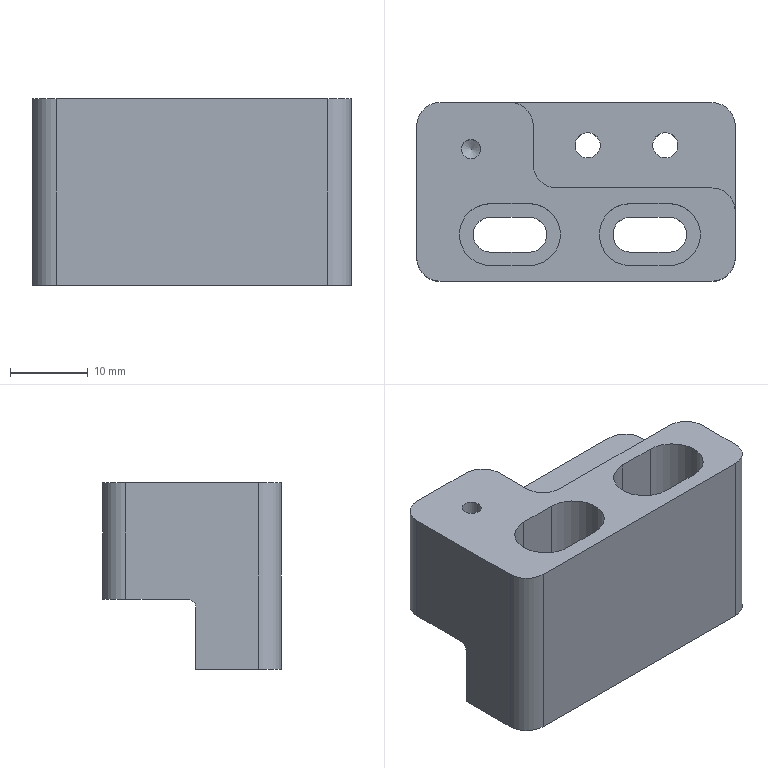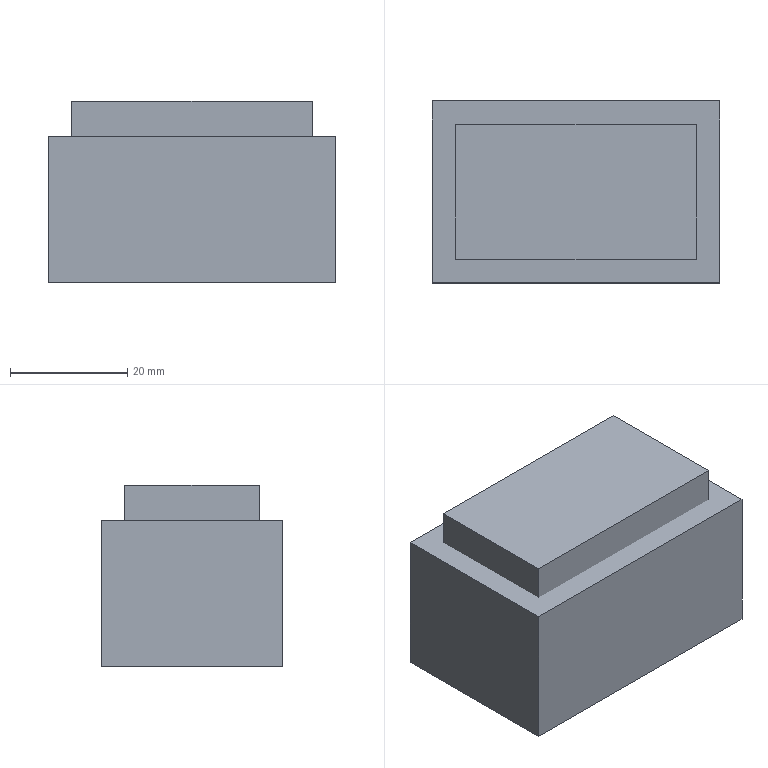CAM job | NX | 3-axis milling, drilling | part box 41 x 23 x 24 mm | stock box 49 x 31 x 31 mm
Tools:
number,name,description,diameter,corner_radius,flute_length,length,flutes
1,D63,Milling Tool-5 Parameters,63.0,0.0,50.0,75.0,2
2,D10,Milling Tool-5 Parameters,10.0,0.0,50.0,75.0,2
9,D6A45,Milling Tool-5 Parameters,6.0,0.0,3.0,3.0,2
16,4.2ZT,Drilling Tool,3.2,0.0,35.0,50.0,2
10,2.5ZT,Drilling Tool,2.4,0.0,35.0,50.0,2
6,D4,Milling Tool-5 Parameters,4.0,0.0,50.0,75.0,2
4,D6,Milling Tool-5 Parameters,6.0,0.0,50.0,75.0,2
Operations:
program,operation,operation_type,tool,method,geometry_group,spindle_rpm,surface_speed,feed_per_tooth,feed_cut,feed_plunge,cut_length_mm,path_length_mm,cut_time_min,machine_time_min
1-45-30-30毛胚,FLOOR_WALL,VolumeBased25DMillingOperation,D63,METHOD,A,6500.0,0.0,0.0,1250.0,100.0,124.0,178.0,0.0992,0.1046
1-45-30-30毛胚,DRILLING,Operation,D6A45,METHOD,A,4000.0,75.0,0.0312,250.0,0.0,12.0,125.625,0.048,0.0594
1-45-30-30毛胚,DRILLING_COPY_1,Operation,4.2ZT,METHOD,A,2000.0,20.0,0.05,200.0,0.0,40.923,155.286,0.2046,0.2161
1-45-30-30毛胚,DRILLING_COPY_1_COPY,Operation,2.5ZT,METHOD,A,2000.0,20.0,0.05,120.0,0.0,11.71,83.42,0.0976,0.1048
1-45-30-30毛胚,ADAPTIVE_MILLING,CavityMilling,D10,METHOD,A,7000.0,219.0,0.1429,2000.0,1000.0,2566.115,2872.667,1.288,1.318
1-45-30-30毛胚,ZLEVEL_PROFILE_COPY_COPY_1_COPY,ZLevelMilling,D10,METHOD,A,6500.0,326.0,0.0769,1000.0,1000.0,326.703,432.362,0.3267,0.3373
1-45-30-30毛胚,CAVITY_MILL_COPY,CavityMilling,D6,METHOD,A,7000.0,87.0,0.0857,1200.0,1000.0,165.753,285.985,0.1456,0.1576
1-45-30-30毛胚,FLOOR_WALL_1_COPY_COPY_1,VolumeBased25DMillingOperation,D6,METHOD,A,7000.0,219.0,0.0714,1000.0,1000.0,198.406,311.367,0.1984,0.2097
1-45-30-30毛胚,ZLEVEL_PROFILE_COPY_COPY_1_COPY_COPY_1,ZLevelMilling,D6,METHOD,A,7000.0,87.0,0.1,1400.0,1000.0,1201.599,1355.55,0.8779,0.8933
1-45-30-30毛胚,ZLEVEL_PROFILE_COPY_COPY_1_COPY_COPY_1_COPY,ZLevelMilling,D4,METHOD,A,7000.0,87.0,0.0929,1300.0,1000.0,1382.52,1583.202,1.079,1.099
1-45-30-30毛胚,ZLEVEL_PROFILE_COPY_1_COPY_COPY_COPY_COPY_COPY_COPY,ZLevelMilling,D6A45,METHOD,A,7000.0,131.0,0.0714,1000.0,1000.0,198.871,517.425,0.1989,0.2307
1-45-30-30毛胚,ZLEVEL_PROFILE_COPY_1_COPY_COPY_COPY_COPY_COPY_COPY_COPY,ZLevelMilling,D6A45,METHOD,A,7000.0,131.0,0.0714,1000.0,1000.0,48.374,304.429,0.0484,0.074
2-45-30-30毛胚,FLOOR_WALL_COPY,VolumeBased25DMillingOperation,D63,METHOD,B,6500.0,0.0,0.0,1250.0,100.0,812.0,1808.002,0.6496,0.7492
2-45-30-30毛胚,ZLEVEL_PROFILE_1_COPY,ZLevelMilling,D10,METHOD,B,7000.0,131.0,0.1786,2500.0,1000.0,534.414,601.314,0.2163,0.2229
2-45-30-30毛胚,ZLEVEL_PROFILE_1_COPY_COPY,ZLevelMilling,D10,METHOD,B,7000.0,131.0,0.1786,2500.0,1000.0,535.78,602.68,0.2168,0.2234
2-45-30-30毛胚,ZLEVEL_PROFILE_COPY_COPY_1_COPY_COPY,ZLevelMilling,D10,METHOD,B,6500.0,326.0,0.0769,1000.0,1000.0,60.081,133.081,0.0601,0.0674
2-45-30-30毛胚,FLOOR_WALL_1_COPY_COPY_1_COPY,VolumeBased25DMillingOperation,D10,METHOD,B,7000.0,219.0,0.0714,1000.0,1000.0,266.206,346.706,0.2662,0.2743
2-45-30-30毛胚,ZLEVEL_PROFILE_1,ZLevelMilling,D10,METHOD,B,7000.0,131.0,0.1786,2500.0,1000.0,1726.211,1800.261,0.6929,0.7003
2-45-30-30毛胚,ZLEVEL_PROFILE_COPY_1_COPY_COPY_COPY_COPY_COPY_COPY_COPY_1,ZLevelMilling,D6A45,METHOD,B,7000.0,131.0,0.0714,1000.0,1000.0,153.671,385.78,0.1537,0.1769
2-45-30-30毛胚,ZLEVEL_PROFILE_COPY_1_COPY_COPY_COPY_COPY_COPY_COPY_COPY_1_COPY,ZLevelMilling,D6A45,METHOD,B,7000.0,131.0,0.0714,1000.0,1000.0,73.946,343.421,0.0739,0.1009